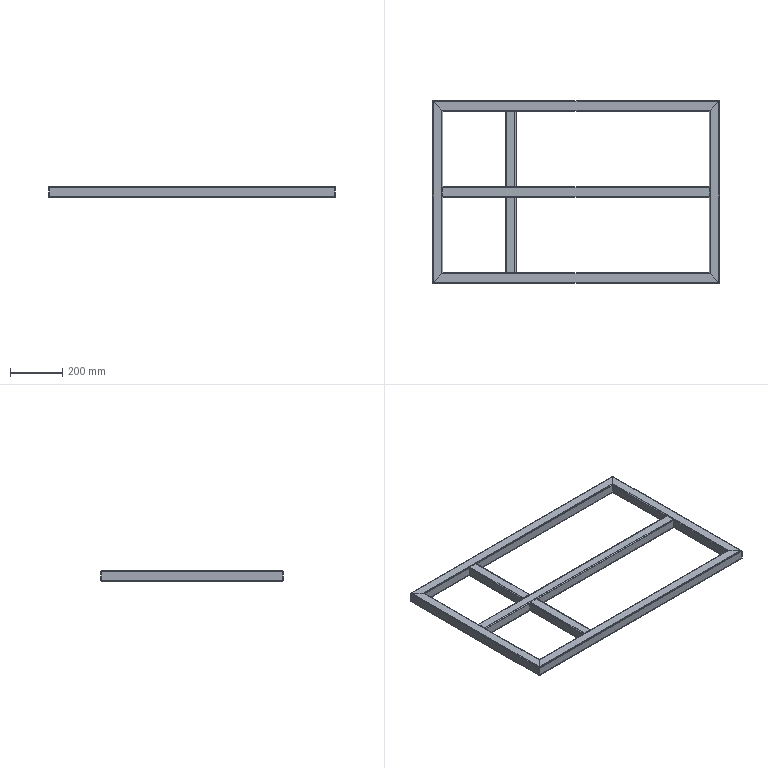Part | SolidWorks | features WeldMemberFeat 1, WeldmentFeature 1 | 7 solids | 126 faces | box 1100 x 700 x 40 mm | volume 1480244 mm3 | plane 70 | cylinder 56 | commonest cylinder face diameters 4 x28 8 x28